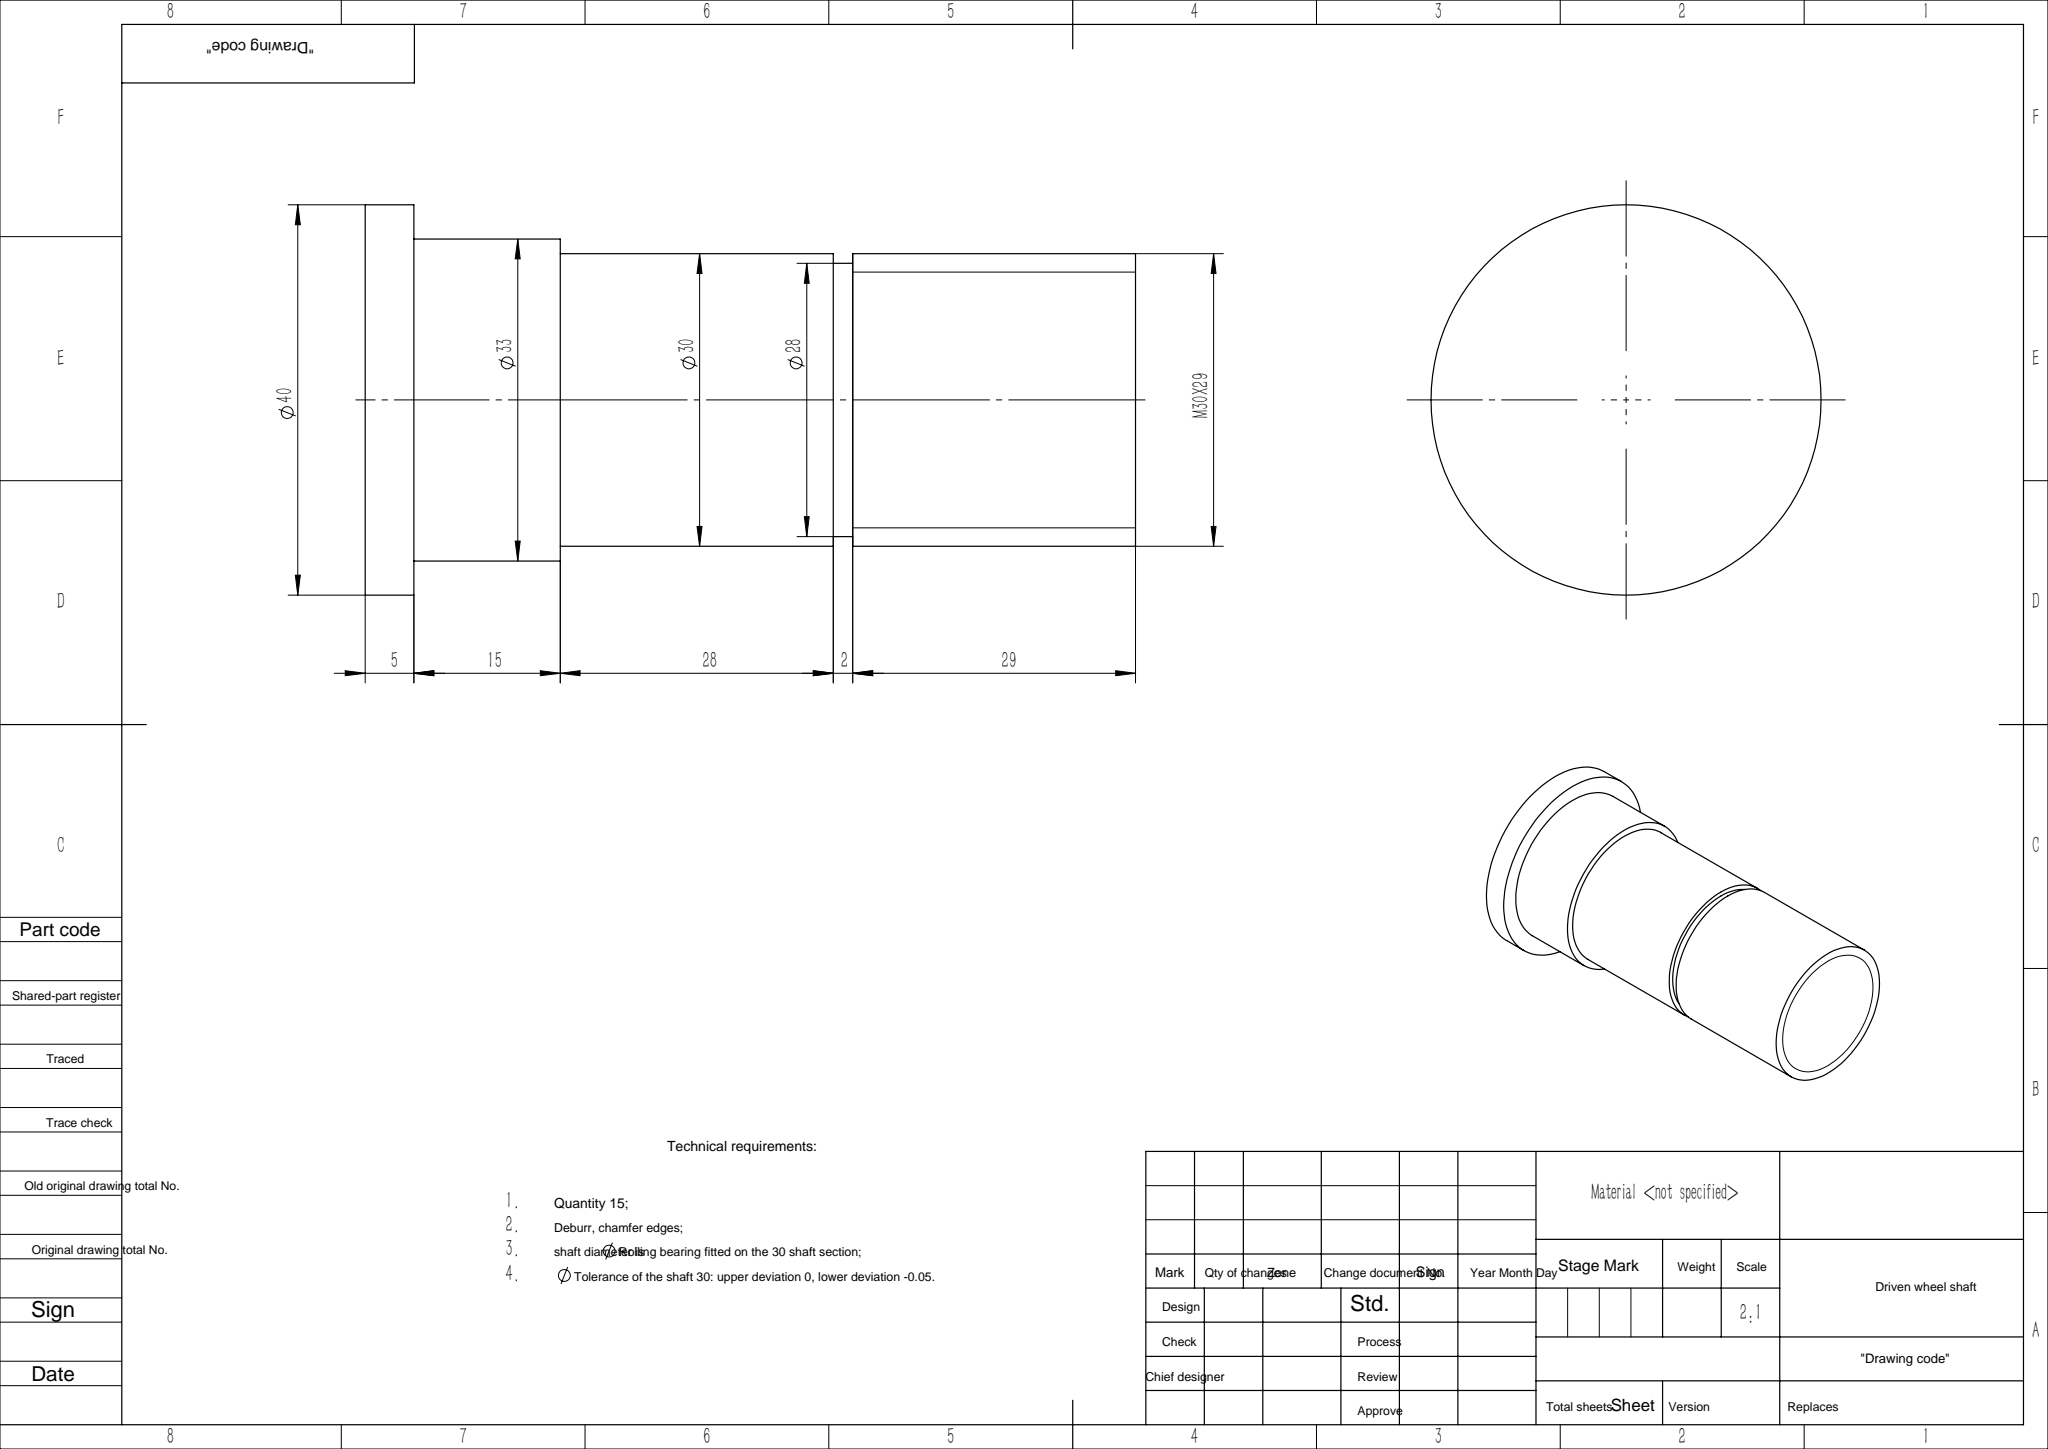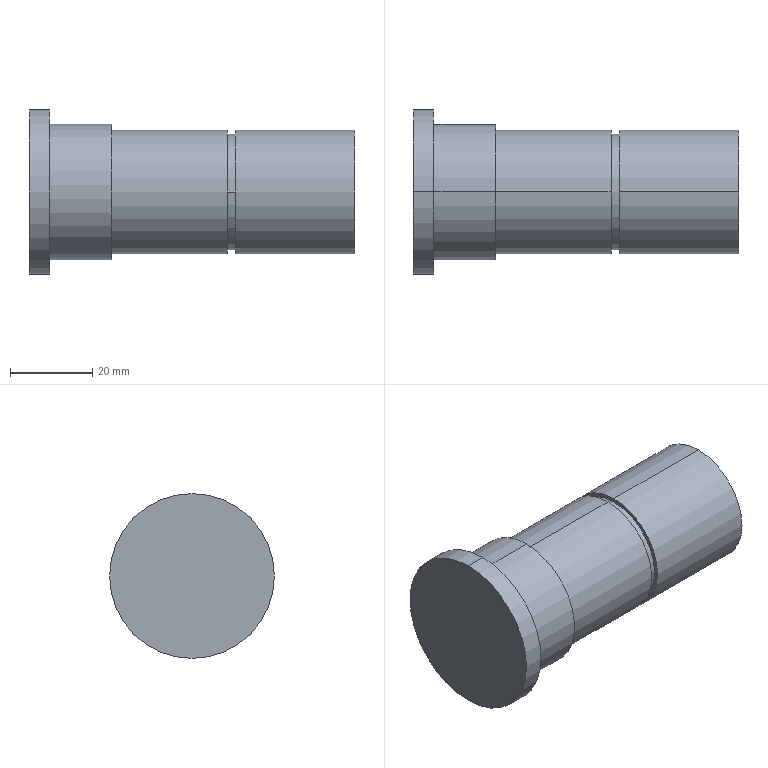Part | SolidWorks | features ICE 1, Revolution 1 | 1 solid | 16 faces | box 79 x 40 x 40 mm | volume 60635 mm3 | cylinder 10 | plane 6 | commonest cylinder face diameters 30 x4 28 x2 33 x2 40 x2
STEP:
#1=CARTESIAN_POINT('',(50.,0.,-15.));
#2=VERTEX_POINT('',#1);
#3=CARTESIAN_POINT('',(50.,0.,15.));
#4=VERTEX_POINT('',#3);
#5=CARTESIAN_POINT('',(50.,0.,0.));
#6=DIRECTION('',(1.,0.,0.));
#7=DIRECTION('',(0.,1.,0.));
#8=AXIS2_PLACEMENT_3D('',#5,#6,#7);
#9=CIRCLE('',#8,15.);
#10=EDGE_CURVE('',#2,#4,#9,.T.);
#11=ORIENTED_EDGE('',*,*,#10,.T.);
#12=CARTESIAN_POINT('',(79.,0.,15.));
#13=VERTEX_POINT('',#12);
#14=CARTESIAN_POINT('',(79.,0.,15.));
#15=DIRECTION('',(1.,0.,0.));
#16=VECTOR('',#15,1000.);
#17=LINE('',#14,#16);
#18=EDGE_CURVE('',#4,#13,#17,.T.);
#19=ORIENTED_EDGE('',*,*,#18,.T.);
#20=CARTESIAN_POINT('',(79.,0.,-15.));
#21=VERTEX_POINT('',#20);
#22=CARTESIAN_POINT('',(79.,0.,0.));
#23=DIRECTION('',(1.,0.,0.));
#24=DIRECTION('',(0.,0.,-1.));
#25=AXIS2_PLACEMENT_3D('',#22,#23,#24);
#26=CIRCLE('',#25,15.);
#27=EDGE_CURVE('',#21,#13,#26,.T.);
#28=ORIENTED_EDGE('',*,*,#27,.F.);
#29=CARTESIAN_POINT('',(79.,0.,-15.));
#30=DIRECTION('',(1.,0.,0.));
#31=VECTOR('',#30,1000.);
#32=LINE('',#29,#31);
#33=EDGE_CURVE('',#2,#21,#32,.T.);
#34=ORIENTED_EDGE('',*,*,#33,.F.);
#35=EDGE_LOOP('',(#11,#19,#28,#34));
#36=FACE_OUTER_BOUND('',#35,.T.);
#37=CARTESIAN_POINT('',(79.,0.,0.));
#38=DIRECTION('',(1.,0.,0.));
#39=DIRECTION('',(0.,0.,-1.));
#40=AXIS2_PLACEMENT_3D('',#37,#38,#39);
#41=CYLINDRICAL_SURFACE('',#40,15.);
#42=ADVANCED_FACE('',(#36),#41,.T.);
#43=CARTESIAN_POINT('',(50.,14.,0.));
#44=VERTEX_POINT('',#43);
#45=CARTESIAN_POINT('',(50.,-14.,0.));
#46=VERTEX_POINT('',#45);
#47=CARTESIAN_POINT('',(50.,0.,0.));
#48=DIRECTION('',(1.,0.,0.));
#49=DIRECTION('',(0.,1.,0.));
#50=AXIS2_PLACEMENT_3D('',#47,#48,#49);
#51=CIRCLE('',#50,14.);
#52=EDGE_CURVE('',#44,#46,#51,.T.);
#53=ORIENTED_EDGE('',*,*,#52,.F.);
#54=CARTESIAN_POINT('',(48.,14.,0.));
#55=VERTEX_POINT('',#54);
#56=CARTESIAN_POINT('',(50.,14.,0.));
#57=DIRECTION('',(-1.,0.,0.));
#58=VECTOR('',#57,1000.);
#59=LINE('',#56,#58);
#60=EDGE_CURVE('',#44,#55,#59,.T.);
#61=ORIENTED_EDGE('',*,*,#60,.T.);
#62=CARTESIAN_POINT('',(48.,-14.,0.));
#63=VERTEX_POINT('',#62);
#64=CARTESIAN_POINT('',(48.,0.,0.));
#65=DIRECTION('',(1.,0.,0.));
#66=DIRECTION('',(0.,1.,0.));
#67=AXIS2_PLACEMENT_3D('',#64,#65,#66);
#68=CIRCLE('',#67,14.);
#69=EDGE_CURVE('',#55,#63,#68,.T.);
#70=ORIENTED_EDGE('',*,*,#69,.T.);
#71=CARTESIAN_POINT('',(50.,-14.,0.));
#72=DIRECTION('',(-1.,0.,0.));
#73=VECTOR('',#72,1000.);
#74=LINE('',#71,#73);
#75=EDGE_CURVE('',#46,#63,#74,.T.);
#76=ORIENTED_EDGE('',*,*,#75,.F.);
#77=EDGE_LOOP('',(#53,#61,#70,#76));
#78=FACE_OUTER_BOUND('',#77,.T.);
#79=CARTESIAN_POINT('',(50.,0.,0.));
#80=DIRECTION('',(-1.,0.,0.));
#81=DIRECTION('',(0.,-1.,0.));
#82=AXIS2_PLACEMENT_3D('',#79,#80,#81);
#83=CYLINDRICAL_SURFACE('',#82,14.);
#84=ADVANCED_FACE('',(#78),#83,.T.);
#85=CARTESIAN_POINT('',(5.,0.,-16.5));
#86=VERTEX_POINT('',#85);
#87=CARTESIAN_POINT('',(5.,0.,16.5));
#88=VERTEX_POINT('',#87);
#89=CARTESIAN_POINT('',(5.,0.,0.));
#90=DIRECTION('',(1.,0.,0.));
#91=DIRECTION('',(0.,0.,-1.));
#92=AXIS2_PLACEMENT_3D('',#89,#90,#91);
#93=CIRCLE('',#92,16.5);
#94=EDGE_CURVE('',#86,#88,#93,.T.);
#95=ORIENTED_EDGE('',*,*,#94,.T.);
#96=CARTESIAN_POINT('',(20.,0.,16.5));
#97=VERTEX_POINT('',#96);
#98=CARTESIAN_POINT('',(79.,0.,16.5));
#99=DIRECTION('',(1.,0.,0.));
#100=VECTOR('',#99,1000.);
#101=LINE('',#98,#100);
#102=EDGE_CURVE('',#88,#97,#101,.T.);
#103=ORIENTED_EDGE('',*,*,#102,.T.);
#104=CARTESIAN_POINT('',(20.,0.,-16.5));
#105=VERTEX_POINT('',#104);
#106=CARTESIAN_POINT('',(20.,0.,0.));
#107=DIRECTION('',(1.,0.,0.));
#108=DIRECTION('',(0.,0.,-1.));
#109=AXIS2_PLACEMENT_3D('',#106,#107,#108);
#110=CIRCLE('',#109,16.5);
#111=EDGE_CURVE('',#105,#97,#110,.T.);
#112=ORIENTED_EDGE('',*,*,#111,.F.);
#113=CARTESIAN_POINT('',(79.,0.,-16.5));
#114=DIRECTION('',(1.,0.,0.));
#115=VECTOR('',#114,1000.);
#116=LINE('',#113,#115);
#117=EDGE_CURVE('',#86,#105,#116,.T.);
#118=ORIENTED_EDGE('',*,*,#117,.F.);
#119=EDGE_LOOP('',(#95,#103,#112,#118));
#120=FACE_OUTER_BOUND('',#119,.T.);
#121=CARTESIAN_POINT('',(79.,0.,0.));
#122=DIRECTION('',(1.,0.,0.));
#123=DIRECTION('',(0.,0.,-1.));
#124=AXIS2_PLACEMENT_3D('',#121,#122,#123);
#125=CYLINDRICAL_SURFACE('',#124,16.5);
#126=ADVANCED_FACE('',(#120),#125,.T.);
#127=CARTESIAN_POINT('',(0.,0.,-20.));
#128=VERTEX_POINT('',#127);
#129=CARTESIAN_POINT('',(0.,0.,20.));
#130=VERTEX_POINT('',#129);
#131=CARTESIAN_POINT('',(0.,0.,0.));
#132=DIRECTION('',(1.,0.,0.));
#133=DIRECTION('',(0.,0.,-1.));
#134=AXIS2_PLACEMENT_3D('',#131,#132,#133);
#135=CIRCLE('',#134,20.);
#136=EDGE_CURVE('',#128,#130,#135,.T.);
#137=ORIENTED_EDGE('',*,*,#136,.T.);
#138=CARTESIAN_POINT('',(5.,0.,20.));
#139=VERTEX_POINT('',#138);
#140=CARTESIAN_POINT('',(79.,0.,20.));
#141=DIRECTION('',(1.,0.,0.));
#142=VECTOR('',#141,1000.);
#143=LINE('',#140,#142);
#144=EDGE_CURVE('',#130,#139,#143,.T.);
#145=ORIENTED_EDGE('',*,*,#144,.T.);
#146=CARTESIAN_POINT('',(5.,0.,-20.));
#147=VERTEX_POINT('',#146);
#148=CARTESIAN_POINT('',(5.,0.,0.));
#149=DIRECTION('',(1.,0.,0.));
#150=DIRECTION('',(0.,0.,-1.));
#151=AXIS2_PLACEMENT_3D('',#148,#149,#150);
#152=CIRCLE('',#151,20.);
#153=EDGE_CURVE('',#147,#139,#152,.T.);
#154=ORIENTED_EDGE('',*,*,#153,.F.);
#155=CARTESIAN_POINT('',(79.,0.,-20.));
#156=DIRECTION('',(1.,0.,0.));
#157=VECTOR('',#156,1000.);
#158=LINE('',#155,#157);
#159=EDGE_CURVE('',#128,#147,#158,.T.);
#160=ORIENTED_EDGE('',*,*,#159,.F.);
#161=EDGE_LOOP('',(#137,#145,#154,#160));
#162=FACE_OUTER_BOUND('',#161,.T.);
#163=CARTESIAN_POINT('',(79.,0.,0.));
#164=DIRECTION('',(1.,0.,0.));
#165=DIRECTION('',(0.,0.,-1.));
#166=AXIS2_PLACEMENT_3D('',#163,#164,#165);
#167=CYLINDRICAL_SURFACE('',#166,20.);
#168=ADVANCED_FACE('',(#162),#167,.T.);
#169=CARTESIAN_POINT('',(20.,0.,-15.));
#170=VERTEX_POINT('',#169);
#171=CARTESIAN_POINT('',(20.,0.,15.));
#172=VERTEX_POINT('',#171);
#173=CARTESIAN_POINT('',(20.,0.,0.));
#174=DIRECTION('',(1.,0.,0.));
#175=DIRECTION('',(0.,0.,-1.));
#176=AXIS2_PLACEMENT_3D('',#173,#174,#175);
#177=CIRCLE('',#176,15.);
#178=EDGE_CURVE('',#170,#172,#177,.T.);
#179=ORIENTED_EDGE('',*,*,#178,.T.);
#180=CARTESIAN_POINT('',(48.,0.,15.));
#181=VERTEX_POINT('',#180);
#182=CARTESIAN_POINT('',(79.,0.,15.));
#183=DIRECTION('',(1.,0.,0.));
#184=VECTOR('',#183,1000.);
#185=LINE('',#182,#184);
#186=EDGE_CURVE('',#172,#181,#185,.T.);
#187=ORIENTED_EDGE('',*,*,#186,.T.);
#188=CARTESIAN_POINT('',(48.,0.,-15.));
#189=VERTEX_POINT('',#188);
#190=CARTESIAN_POINT('',(48.,0.,0.));
#191=DIRECTION('',(1.,0.,0.));
#192=DIRECTION('',(0.,1.,0.));
#193=AXIS2_PLACEMENT_3D('',#190,#191,#192);
#194=CIRCLE('',#193,15.);
#195=EDGE_CURVE('',#189,#181,#194,.T.);
#196=ORIENTED_EDGE('',*,*,#195,.F.);
#197=CARTESIAN_POINT('',(79.,0.,-15.));
#198=DIRECTION('',(1.,0.,0.));
#199=VECTOR('',#198,1000.);
#200=LINE('',#197,#199);
#201=EDGE_CURVE('',#170,#189,#200,.T.);
#202=ORIENTED_EDGE('',*,*,#201,.F.);
#203=EDGE_LOOP('',(#179,#187,#196,#202));
#204=FACE_OUTER_BOUND('',#203,.T.);
#205=CARTESIAN_POINT('',(79.,0.,0.));
#206=DIRECTION('',(1.,0.,0.));
#207=DIRECTION('',(0.,0.,-1.));
#208=AXIS2_PLACEMENT_3D('',#205,#206,#207);
#209=CYLINDRICAL_SURFACE('',#208,15.);
#210=ADVANCED_FACE('',(#204),#209,.T.);
#211=ORIENTED_EDGE('',*,*,#186,.F.);
#212=CARTESIAN_POINT('',(20.,0.,0.));
#213=DIRECTION('',(1.,0.,0.));
#214=DIRECTION('',(0.,0.,-1.));
#215=AXIS2_PLACEMENT_3D('',#212,#213,#214);
#216=CIRCLE('',#215,15.);
#217=EDGE_CURVE('',#172,#170,#216,.T.);
#218=ORIENTED_EDGE('',*,*,#217,.T.);
#219=ORIENTED_EDGE('',*,*,#201,.T.);
#220=CARTESIAN_POINT('',(48.,0.,0.));
#221=DIRECTION('',(1.,0.,0.));
#222=DIRECTION('',(0.,1.,0.));
#223=AXIS2_PLACEMENT_3D('',#220,#221,#222);
#224=CIRCLE('',#223,15.);
#225=EDGE_CURVE('',#181,#189,#224,.T.);
#226=ORIENTED_EDGE('',*,*,#225,.F.);
#227=EDGE_LOOP('',(#211,#218,#219,#226));
#228=FACE_OUTER_BOUND('',#227,.T.);
#229=CARTESIAN_POINT('',(79.,0.,0.));
#230=DIRECTION('',(1.,0.,0.));
#231=DIRECTION('',(0.,0.,-1.));
#232=AXIS2_PLACEMENT_3D('',#229,#230,#231);
#233=CYLINDRICAL_SURFACE('',#232,15.);
#234=ADVANCED_FACE('',(#228),#233,.T.);
#235=ORIENTED_EDGE('',*,*,#136,.F.);
#236=CARTESIAN_POINT('',(0.,0.,0.));
#237=DIRECTION('',(1.,0.,0.));
#238=DIRECTION('',(0.,0.,-1.));
#239=AXIS2_PLACEMENT_3D('',#236,#237,#238);
#240=CIRCLE('',#239,20.);
#241=EDGE_CURVE('',#130,#128,#240,.T.);
#242=ORIENTED_EDGE('',*,*,#241,.F.);
#243=EDGE_LOOP('',(#235,#242));
#244=FACE_OUTER_BOUND('',#243,.T.);
#245=CARTESIAN_POINT('',(0.,0.,0.));
#246=DIRECTION('',(-1.,0.,0.));
#247=DIRECTION('',(0.,0.,1.));
#248=AXIS2_PLACEMENT_3D('',#245,#246,#247);
#249=PLANE('',#248);
#250=ADVANCED_FACE('',(#244),#249,.T.);
#251=ORIENTED_EDGE('',*,*,#144,.F.);
#252=ORIENTED_EDGE('',*,*,#241,.T.);
#253=ORIENTED_EDGE('',*,*,#159,.T.);
#254=CARTESIAN_POINT('',(5.,0.,0.));
#255=DIRECTION('',(1.,0.,0.));
#256=DIRECTION('',(0.,0.,-1.));
#257=AXIS2_PLACEMENT_3D('',#254,#255,#256);
#258=CIRCLE('',#257,20.);
#259=EDGE_CURVE('',#139,#147,#258,.T.);
#260=ORIENTED_EDGE('',*,*,#259,.F.);
#261=EDGE_LOOP('',(#251,#252,#253,#260));
#262=FACE_OUTER_BOUND('',#261,.T.);
#263=CARTESIAN_POINT('',(79.,0.,0.));
#264=DIRECTION('',(1.,0.,0.));
#265=DIRECTION('',(0.,0.,-1.));
#266=AXIS2_PLACEMENT_3D('',#263,#264,#265);
#267=CYLINDRICAL_SURFACE('',#266,20.);
#268=ADVANCED_FACE('',(#262),#267,.T.);
#269=ORIENTED_EDGE('',*,*,#153,.T.);
#270=ORIENTED_EDGE('',*,*,#259,.T.);
#271=EDGE_LOOP('',(#269,#270));
#272=FACE_OUTER_BOUND('',#271,.T.);
#273=ORIENTED_EDGE('',*,*,#94,.F.);
#274=CARTESIAN_POINT('',(5.,0.,0.));
#275=DIRECTION('',(1.,0.,0.));
#276=DIRECTION('',(0.,0.,-1.));
#277=AXIS2_PLACEMENT_3D('',#274,#275,#276);
#278=CIRCLE('',#277,16.5);
#279=EDGE_CURVE('',#88,#86,#278,.T.);
#280=ORIENTED_EDGE('',*,*,#279,.F.);
#281=EDGE_LOOP('',(#273,#280));
#282=FACE_BOUND('',#281,.T.);
#283=CARTESIAN_POINT('',(5.,20.,0.));
#284=DIRECTION('',(1.,0.,0.));
#285=DIRECTION('',(0.,0.,-1.));
#286=AXIS2_PLACEMENT_3D('',#283,#284,#285);
#287=PLANE('',#286);
#288=ADVANCED_FACE('',(#272,#282),#287,.T.);
#289=ORIENTED_EDGE('',*,*,#102,.F.);
#290=ORIENTED_EDGE('',*,*,#279,.T.);
#291=ORIENTED_EDGE('',*,*,#117,.T.);
#292=CARTESIAN_POINT('',(20.,0.,0.));
#293=DIRECTION('',(1.,0.,0.));
#294=DIRECTION('',(0.,0.,-1.));
#295=AXIS2_PLACEMENT_3D('',#292,#293,#294);
#296=CIRCLE('',#295,16.5);
#297=EDGE_CURVE('',#97,#105,#296,.T.);
#298=ORIENTED_EDGE('',*,*,#297,.F.);
#299=EDGE_LOOP('',(#289,#290,#291,#298));
#300=FACE_OUTER_BOUND('',#299,.T.);
#301=CARTESIAN_POINT('',(79.,0.,0.));
#302=DIRECTION('',(1.,0.,0.));
#303=DIRECTION('',(0.,0.,-1.));
#304=AXIS2_PLACEMENT_3D('',#301,#302,#303);
#305=CYLINDRICAL_SURFACE('',#304,16.5);
#306=ADVANCED_FACE('',(#300),#305,.T.);
#307=ORIENTED_EDGE('',*,*,#111,.T.);
#308=ORIENTED_EDGE('',*,*,#297,.T.);
#309=EDGE_LOOP('',(#307,#308));
#310=FACE_OUTER_BOUND('',#309,.T.);
#311=ORIENTED_EDGE('',*,*,#178,.F.);
#312=ORIENTED_EDGE('',*,*,#217,.F.);
#313=EDGE_LOOP('',(#311,#312));
#314=FACE_BOUND('',#313,.T.);
#315=CARTESIAN_POINT('',(20.,16.5,0.));
#316=DIRECTION('',(1.,0.,0.));
#317=DIRECTION('',(0.,0.,-1.));
#318=AXIS2_PLACEMENT_3D('',#315,#316,#317);
#319=PLANE('',#318);
#320=ADVANCED_FACE('',(#310,#314),#319,.T.);
#321=ORIENTED_EDGE('',*,*,#10,.F.);
#322=CARTESIAN_POINT('',(50.,0.,0.));
#323=DIRECTION('',(1.,0.,0.));
#324=DIRECTION('',(0.,1.,0.));
#325=AXIS2_PLACEMENT_3D('',#322,#323,#324);
#326=CIRCLE('',#325,15.);
#327=EDGE_CURVE('',#4,#2,#326,.T.);
#328=ORIENTED_EDGE('',*,*,#327,.F.);
#329=EDGE_LOOP('',(#321,#328));
#330=FACE_OUTER_BOUND('',#329,.T.);
#331=CARTESIAN_POINT('',(50.,0.,0.));
#332=DIRECTION('',(1.,0.,0.));
#333=DIRECTION('',(0.,1.,0.));
#334=AXIS2_PLACEMENT_3D('',#331,#332,#333);
#335=CIRCLE('',#334,14.);
#336=EDGE_CURVE('',#46,#44,#335,.T.);
#337=ORIENTED_EDGE('',*,*,#336,.T.);
#338=ORIENTED_EDGE('',*,*,#52,.T.);
#339=EDGE_LOOP('',(#337,#338));
#340=FACE_BOUND('',#339,.T.);
#341=CARTESIAN_POINT('',(50.,0.,0.));
#342=DIRECTION('',(1.,0.,0.));
#343=DIRECTION('',(0.,1.,0.));
#344=AXIS2_PLACEMENT_3D('',#341,#342,#343);
#345=PLANE('',#344);
#346=ADVANCED_FACE('',(#330,#340),#345,.F.);
#347=ORIENTED_EDGE('',*,*,#195,.T.);
#348=ORIENTED_EDGE('',*,*,#225,.T.);
#349=EDGE_LOOP('',(#347,#348));
#350=FACE_OUTER_BOUND('',#349,.T.);
#351=CARTESIAN_POINT('',(48.,0.,0.));
#352=DIRECTION('',(1.,0.,0.));
#353=DIRECTION('',(0.,1.,0.));
#354=AXIS2_PLACEMENT_3D('',#351,#352,#353);
#355=CIRCLE('',#354,14.);
#356=EDGE_CURVE('',#63,#55,#355,.T.);
#357=ORIENTED_EDGE('',*,*,#356,.F.);
#358=ORIENTED_EDGE('',*,*,#69,.F.);
#359=EDGE_LOOP('',(#357,#358));
#360=FACE_BOUND('',#359,.T.);
#361=CARTESIAN_POINT('',(48.,0.,0.));
#362=DIRECTION('',(1.,0.,0.));
#363=DIRECTION('',(0.,1.,0.));
#364=AXIS2_PLACEMENT_3D('',#361,#362,#363);
#365=PLANE('',#364);
#366=ADVANCED_FACE('',(#350,#360),#365,.T.);
#367=ORIENTED_EDGE('',*,*,#60,.F.);
#368=ORIENTED_EDGE('',*,*,#336,.F.);
#369=ORIENTED_EDGE('',*,*,#75,.T.);
#370=ORIENTED_EDGE('',*,*,#356,.T.);
#371=EDGE_LOOP('',(#367,#368,#369,#370));
#372=FACE_OUTER_BOUND('',#371,.T.);
#373=CARTESIAN_POINT('',(50.,0.,0.));
#374=DIRECTION('',(-1.,0.,0.));
#375=DIRECTION('',(0.,-1.,0.));
#376=AXIS2_PLACEMENT_3D('',#373,#374,#375);
#377=CYLINDRICAL_SURFACE('',#376,14.);
#378=ADVANCED_FACE('',(#372),#377,.T.);
#379=ORIENTED_EDGE('',*,*,#27,.T.);
#380=CARTESIAN_POINT('',(79.,0.,0.));
#381=DIRECTION('',(1.,0.,0.));
#382=DIRECTION('',(0.,0.,-1.));
#383=AXIS2_PLACEMENT_3D('',#380,#381,#382);
#384=CIRCLE('',#383,15.);
#385=EDGE_CURVE('',#13,#21,#384,.T.);
#386=ORIENTED_EDGE('',*,*,#385,.T.);
#387=EDGE_LOOP('',(#379,#386));
#388=FACE_OUTER_BOUND('',#387,.T.);
#389=CARTESIAN_POINT('',(79.,15.,0.));
#390=DIRECTION('',(1.,0.,0.));
#391=DIRECTION('',(0.,0.,-1.));
#392=AXIS2_PLACEMENT_3D('',#389,#390,#391);
#393=PLANE('',#392);
#394=ADVANCED_FACE('',(#388),#393,.T.);
#395=ORIENTED_EDGE('',*,*,#18,.F.);
#396=ORIENTED_EDGE('',*,*,#327,.T.);
#397=ORIENTED_EDGE('',*,*,#33,.T.);
#398=ORIENTED_EDGE('',*,*,#385,.F.);
#399=EDGE_LOOP('',(#395,#396,#397,#398));
#400=FACE_OUTER_BOUND('',#399,.T.);
#401=CARTESIAN_POINT('',(79.,0.,0.));
#402=DIRECTION('',(1.,0.,0.));
#403=DIRECTION('',(0.,0.,-1.));
#404=AXIS2_PLACEMENT_3D('',#401,#402,#403);
#405=CYLINDRICAL_SURFACE('',#404,15.);
#406=ADVANCED_FACE('',(#400),#405,.T.);
#407=CLOSED_SHELL('',(#42,#84,#126,#168,#210,#234,#250,#268,#288,#306,#320,#346,#366,#378,#394,#406));
#408=MANIFOLD_SOLID_BREP('',#407);
#409=CARTESIAN_POINT('',(0.,0.,0.));
#410=DIRECTION('',(0.,0.,1.));
#411=DIRECTION('',(1.,0.,0.));
#412=AXIS2_PLACEMENT_3D('',#409,#410,#411);
#413=(LENGTH_UNIT()NAMED_UNIT(*)SI_UNIT(.MILLI.,.METRE.));
#414=UNCERTAINTY_MEASURE_WITH_UNIT(LENGTH_MEASURE(0.00001),#413,'','');
#415=(NAMED_UNIT(*)PLANE_ANGLE_UNIT()SI_UNIT($,.RADIAN.));
#416=(NAMED_UNIT(*)SI_UNIT($,.STERADIAN.)SOLID_ANGLE_UNIT());
#417=(GEOMETRIC_REPRESENTATION_CONTEXT(3)GLOBAL_UNCERTAINTY_ASSIGNED_CONTEXT((#414))GLOBAL_UNIT_ASSIGNED_CONTEXT((#413,#415,#416))REPRESENTATION_CONTEXT('',''));
#418=ADVANCED_BREP_SHAPE_REPRESENTATION('',(#408,#412),#417);